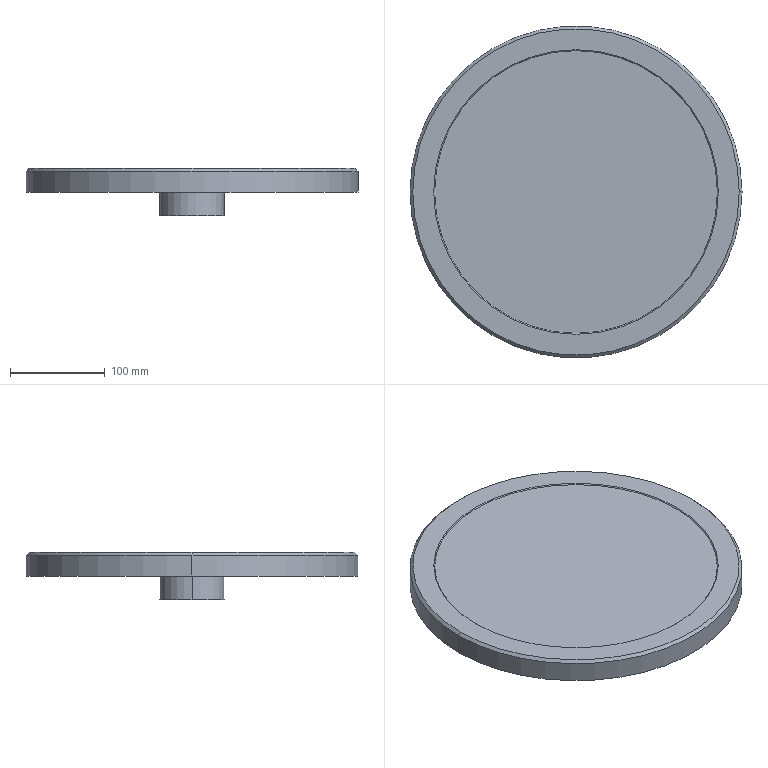Part | SolidWorks | features ICE 2, Chamfer 1, Extrusion 1, Fillet 1 | 1 solid | 14 faces | box 350 x 350 x 50 mm | volume 2420950 mm3 | cone 4 | cylinder 4 | plane 4 | torus 2 | commonest cylinder face diameters 68 x2 350 x2
STEP:
#1=CARTESIAN_POINT('',(172.,0.,50.));
#2=VERTEX_POINT('',#1);
#3=CARTESIAN_POINT('',(-172.,0.,50.));
#4=VERTEX_POINT('',#3);
#5=CARTESIAN_POINT('',(0.,0.,50.));
#6=DIRECTION('',(0.,0.,1.));
#7=DIRECTION('',(1.,0.,0.));
#8=AXIS2_PLACEMENT_3D('',#5,#6,#7);
#9=CIRCLE('',#8,172.);
#10=EDGE_CURVE('',#2,#4,#9,.T.);
#11=ORIENTED_EDGE('',*,*,#10,.F.);
#12=CARTESIAN_POINT('',(175.,0.,47.));
#13=VERTEX_POINT('',#12);
#14=CARTESIAN_POINT('',(172.,0.,50.));
#15=DIRECTION('',(0.7071,0.,-0.7071));
#16=VECTOR('',#15,1000.);
#17=LINE('',#14,#16);
#18=EDGE_CURVE('',#2,#13,#17,.T.);
#19=ORIENTED_EDGE('',*,*,#18,.T.);
#20=CARTESIAN_POINT('',(-175.,0.,47.));
#21=VERTEX_POINT('',#20);
#22=CARTESIAN_POINT('',(0.,0.,47.));
#23=DIRECTION('',(0.,0.,-1.));
#24=DIRECTION('',(1.,0.,0.));
#25=AXIS2_PLACEMENT_3D('',#22,#23,#24);
#26=CIRCLE('',#25,175.);
#27=EDGE_CURVE('',#21,#13,#26,.T.);
#28=ORIENTED_EDGE('',*,*,#27,.F.);
#29=CARTESIAN_POINT('',(-172.,0.,50.));
#30=DIRECTION('',(-0.7071,0.,-0.7071));
#31=VECTOR('',#30,1000.);
#32=LINE('',#29,#31);
#33=EDGE_CURVE('',#4,#21,#32,.T.);
#34=ORIENTED_EDGE('',*,*,#33,.F.);
#35=EDGE_LOOP('',(#11,#19,#28,#34));
#36=FACE_OUTER_BOUND('',#35,.T.);
#37=CARTESIAN_POINT('',(0.,0.,50.));
#38=DIRECTION('',(0.,0.,-1.));
#39=DIRECTION('',(-1.,0.,0.));
#40=AXIS2_PLACEMENT_3D('',#37,#38,#39);
#41=CONICAL_SURFACE('',#40,172.,0.7854);
#42=ADVANCED_FACE('',(#36),#41,.T.);
#43=CARTESIAN_POINT('',(-34.5,0.,25.));
#44=VERTEX_POINT('',#43);
#45=CARTESIAN_POINT('',(34.5,0.,25.));
#46=VERTEX_POINT('',#45);
#47=CARTESIAN_POINT('',(0.,0.,25.));
#48=DIRECTION('',(0.,0.,1.));
#49=DIRECTION('',(1.,0.,0.));
#50=AXIS2_PLACEMENT_3D('',#47,#48,#49);
#51=CIRCLE('',#50,34.5);
#52=EDGE_CURVE('',#44,#46,#51,.T.);
#53=ORIENTED_EDGE('',*,*,#52,.F.);
#54=CARTESIAN_POINT('',(-34.,0.,24.5));
#55=VERTEX_POINT('',#54);
#56=CARTESIAN_POINT('',(-34.5,0.,24.5));
#57=DIRECTION('',(0.,1.,0.));
#58=DIRECTION('',(-1.,0.,0.));
#59=AXIS2_PLACEMENT_3D('',#56,#57,#58);
#60=CIRCLE('',#59,0.5);
#61=EDGE_CURVE('',#44,#55,#60,.T.);
#62=ORIENTED_EDGE('',*,*,#61,.T.);
#63=CARTESIAN_POINT('',(34.,0.,24.5));
#64=VERTEX_POINT('',#63);
#65=CARTESIAN_POINT('',(0.,0.,24.5));
#66=DIRECTION('',(0.,0.,-1.));
#67=DIRECTION('',(1.,0.,0.));
#68=AXIS2_PLACEMENT_3D('',#65,#66,#67);
#69=CIRCLE('',#68,34.);
#70=EDGE_CURVE('',#64,#55,#69,.T.);
#71=ORIENTED_EDGE('',*,*,#70,.F.);
#72=CARTESIAN_POINT('',(34.5,0.,24.5));
#73=DIRECTION('',(0.,-1.,0.));
#74=DIRECTION('',(0.,0.,-1.));
#75=AXIS2_PLACEMENT_3D('',#72,#73,#74);
#76=CIRCLE('',#75,0.5);
#77=EDGE_CURVE('',#46,#64,#76,.T.);
#78=ORIENTED_EDGE('',*,*,#77,.F.);
#79=EDGE_LOOP('',(#53,#62,#71,#78));
#80=FACE_OUTER_BOUND('',#79,.T.);
#81=CARTESIAN_POINT('',(0.,0.,24.5));
#82=DIRECTION('',(0.,0.,1.));
#83=DIRECTION('',(1.,0.,0.));
#84=AXIS2_PLACEMENT_3D('',#81,#82,#83);
#85=TOROIDAL_SURFACE('',#84,34.5,0.5);
#86=ADVANCED_FACE('',(#80),#85,.F.);
#87=CARTESIAN_POINT('',(-149.,0.,49.));
#88=VERTEX_POINT('',#87);
#89=CARTESIAN_POINT('',(149.,0.,49.));
#90=VERTEX_POINT('',#89);
#91=CARTESIAN_POINT('',(0.,0.,49.));
#92=DIRECTION('',(0.,0.,1.));
#93=DIRECTION('',(1.,0.,0.));
#94=AXIS2_PLACEMENT_3D('',#91,#92,#93);
#95=CIRCLE('',#94,149.);
#96=EDGE_CURVE('',#88,#90,#95,.T.);
#97=ORIENTED_EDGE('',*,*,#96,.F.);
#98=CARTESIAN_POINT('',(-150.,0.,50.));
#99=VERTEX_POINT('',#98);
#100=CARTESIAN_POINT('',(-150.,0.,50.));
#101=DIRECTION('',(-0.7071,0.,0.7071));
#102=VECTOR('',#101,1000.);
#103=LINE('',#100,#102);
#104=EDGE_CURVE('',#88,#99,#103,.T.);
#105=ORIENTED_EDGE('',*,*,#104,.T.);
#106=CARTESIAN_POINT('',(150.,0.,50.));
#107=VERTEX_POINT('',#106);
#108=CARTESIAN_POINT('',(0.,0.,50.));
#109=DIRECTION('',(0.,0.,1.));
#110=DIRECTION('',(1.,0.,0.));
#111=AXIS2_PLACEMENT_3D('',#108,#109,#110);
#112=CIRCLE('',#111,150.);
#113=EDGE_CURVE('',#99,#107,#112,.T.);
#114=ORIENTED_EDGE('',*,*,#113,.T.);
#115=CARTESIAN_POINT('',(150.,0.,50.));
#116=DIRECTION('',(0.7071,0.,0.7071));
#117=VECTOR('',#116,1000.);
#118=LINE('',#115,#117);
#119=EDGE_CURVE('',#90,#107,#118,.T.);
#120=ORIENTED_EDGE('',*,*,#119,.F.);
#121=EDGE_LOOP('',(#97,#105,#114,#120));
#122=FACE_OUTER_BOUND('',#121,.T.);
#123=CARTESIAN_POINT('',(0.,0.,50.));
#124=DIRECTION('',(0.,0.,1.));
#125=DIRECTION('',(1.,0.,0.));
#126=AXIS2_PLACEMENT_3D('',#123,#124,#125);
#127=CONICAL_SURFACE('',#126,150.,0.7854);
#128=ADVANCED_FACE('',(#122),#127,.F.);
#129=CARTESIAN_POINT('',(175.,0.,25.));
#130=VERTEX_POINT('',#129);
#131=CARTESIAN_POINT('',(-175.,0.,25.));
#132=VERTEX_POINT('',#131);
#133=CARTESIAN_POINT('',(0.,0.,25.));
#134=DIRECTION('',(0.,0.,1.));
#135=DIRECTION('',(1.,0.,0.));
#136=AXIS2_PLACEMENT_3D('',#133,#134,#135);
#137=CIRCLE('',#136,175.);
#138=EDGE_CURVE('',#130,#132,#137,.T.);
#139=ORIENTED_EDGE('',*,*,#138,.T.);
#140=CARTESIAN_POINT('',(-175.,0.,25.));
#141=DIRECTION('',(0.,0.,1.));
#142=VECTOR('',#141,1000.);
#143=LINE('',#140,#142);
#144=EDGE_CURVE('',#132,#21,#143,.T.);
#145=ORIENTED_EDGE('',*,*,#144,.T.);
#146=ORIENTED_EDGE('',*,*,#27,.T.);
#147=CARTESIAN_POINT('',(175.,0.,25.));
#148=DIRECTION('',(0.,0.,1.));
#149=VECTOR('',#148,1000.);
#150=LINE('',#147,#149);
#151=EDGE_CURVE('',#130,#13,#150,.T.);
#152=ORIENTED_EDGE('',*,*,#151,.F.);
#153=EDGE_LOOP('',(#139,#145,#146,#152));
#154=FACE_OUTER_BOUND('',#153,.T.);
#155=CARTESIAN_POINT('',(0.,0.,25.));
#156=DIRECTION('',(0.,0.,1.));
#157=DIRECTION('',(1.,0.,0.));
#158=AXIS2_PLACEMENT_3D('',#155,#156,#157);
#159=CYLINDRICAL_SURFACE('',#158,175.);
#160=ADVANCED_FACE('',(#154),#159,.T.);
#161=CARTESIAN_POINT('',(0.,0.,24.5));
#162=DIRECTION('',(0.,0.,-1.));
#163=DIRECTION('',(1.,0.,0.));
#164=AXIS2_PLACEMENT_3D('',#161,#162,#163);
#165=CIRCLE('',#164,34.);
#166=EDGE_CURVE('',#55,#64,#165,.T.);
#167=ORIENTED_EDGE('',*,*,#166,.T.);
#168=CARTESIAN_POINT('',(34.,0.,0.));
#169=VERTEX_POINT('',#168);
#170=CARTESIAN_POINT('',(34.,0.,50.));
#171=DIRECTION('',(0.,0.,-1.));
#172=VECTOR('',#171,1000.);
#173=LINE('',#170,#172);
#174=EDGE_CURVE('',#64,#169,#173,.T.);
#175=ORIENTED_EDGE('',*,*,#174,.T.);
#176=CARTESIAN_POINT('',(-34.,0.,0.));
#177=VERTEX_POINT('',#176);
#178=CARTESIAN_POINT('',(0.,0.,0.));
#179=DIRECTION('',(0.,0.,1.));
#180=DIRECTION('',(1.,0.,0.));
#181=AXIS2_PLACEMENT_3D('',#178,#179,#180);
#182=CIRCLE('',#181,34.);
#183=EDGE_CURVE('',#169,#177,#182,.T.);
#184=ORIENTED_EDGE('',*,*,#183,.T.);
#185=CARTESIAN_POINT('',(-34.,0.,50.));
#186=DIRECTION('',(0.,0.,-1.));
#187=VECTOR('',#186,1000.);
#188=LINE('',#185,#187);
#189=EDGE_CURVE('',#55,#177,#188,.T.);
#190=ORIENTED_EDGE('',*,*,#189,.F.);
#191=EDGE_LOOP('',(#167,#175,#184,#190));
#192=FACE_OUTER_BOUND('',#191,.T.);
#193=CARTESIAN_POINT('',(0.,0.,50.));
#194=DIRECTION('',(0.,0.,-1.));
#195=DIRECTION('',(-1.,0.,0.));
#196=AXIS2_PLACEMENT_3D('',#193,#194,#195);
#197=CYLINDRICAL_SURFACE('',#196,34.);
#198=ADVANCED_FACE('',(#192),#197,.T.);
#199=ORIENTED_EDGE('',*,*,#174,.F.);
#200=ORIENTED_EDGE('',*,*,#70,.T.);
#201=ORIENTED_EDGE('',*,*,#189,.T.);
#202=CARTESIAN_POINT('',(0.,0.,0.));
#203=DIRECTION('',(0.,0.,1.));
#204=DIRECTION('',(1.,0.,0.));
#205=AXIS2_PLACEMENT_3D('',#202,#203,#204);
#206=CIRCLE('',#205,34.);
#207=EDGE_CURVE('',#177,#169,#206,.T.);
#208=ORIENTED_EDGE('',*,*,#207,.T.);
#209=EDGE_LOOP('',(#199,#200,#201,#208));
#210=FACE_OUTER_BOUND('',#209,.T.);
#211=CARTESIAN_POINT('',(0.,0.,50.));
#212=DIRECTION('',(0.,0.,-1.));
#213=DIRECTION('',(-1.,0.,0.));
#214=AXIS2_PLACEMENT_3D('',#211,#212,#213);
#215=CYLINDRICAL_SURFACE('',#214,34.);
#216=ADVANCED_FACE('',(#210),#215,.T.);
#217=ORIENTED_EDGE('',*,*,#207,.F.);
#218=ORIENTED_EDGE('',*,*,#183,.F.);
#219=EDGE_LOOP('',(#217,#218));
#220=FACE_OUTER_BOUND('',#219,.T.);
#221=CARTESIAN_POINT('',(0.,0.,0.));
#222=DIRECTION('',(0.,0.,1.));
#223=DIRECTION('',(1.,0.,0.));
#224=AXIS2_PLACEMENT_3D('',#221,#222,#223);
#225=PLANE('',#224);
#226=ADVANCED_FACE('',(#220),#225,.F.);
#227=ORIENTED_EDGE('',*,*,#144,.F.);
#228=CARTESIAN_POINT('',(0.,0.,25.));
#229=DIRECTION('',(0.,0.,1.));
#230=DIRECTION('',(1.,0.,0.));
#231=AXIS2_PLACEMENT_3D('',#228,#229,#230);
#232=CIRCLE('',#231,175.);
#233=EDGE_CURVE('',#132,#130,#232,.T.);
#234=ORIENTED_EDGE('',*,*,#233,.T.);
#235=ORIENTED_EDGE('',*,*,#151,.T.);
#236=CARTESIAN_POINT('',(0.,0.,47.));
#237=DIRECTION('',(0.,0.,-1.));
#238=DIRECTION('',(1.,0.,0.));
#239=AXIS2_PLACEMENT_3D('',#236,#237,#238);
#240=CIRCLE('',#239,175.);
#241=EDGE_CURVE('',#13,#21,#240,.T.);
#242=ORIENTED_EDGE('',*,*,#241,.T.);
#243=EDGE_LOOP('',(#227,#234,#235,#242));
#244=FACE_OUTER_BOUND('',#243,.T.);
#245=CARTESIAN_POINT('',(0.,0.,25.));
#246=DIRECTION('',(0.,0.,1.));
#247=DIRECTION('',(1.,0.,0.));
#248=AXIS2_PLACEMENT_3D('',#245,#246,#247);
#249=CYLINDRICAL_SURFACE('',#248,175.);
#250=ADVANCED_FACE('',(#244),#249,.T.);
#251=CARTESIAN_POINT('',(0.,0.,25.));
#252=DIRECTION('',(0.,0.,1.));
#253=DIRECTION('',(1.,0.,0.));
#254=AXIS2_PLACEMENT_3D('',#251,#252,#253);
#255=CIRCLE('',#254,34.5);
#256=EDGE_CURVE('',#46,#44,#255,.T.);
#257=ORIENTED_EDGE('',*,*,#256,.T.);
#258=ORIENTED_EDGE('',*,*,#52,.T.);
#259=EDGE_LOOP('',(#257,#258));
#260=FACE_BOUND('',#259,.T.);
#261=ORIENTED_EDGE('',*,*,#138,.F.);
#262=ORIENTED_EDGE('',*,*,#233,.F.);
#263=EDGE_LOOP('',(#261,#262));
#264=FACE_OUTER_BOUND('',#263,.T.);
#265=CARTESIAN_POINT('',(0.,0.,25.));
#266=DIRECTION('',(0.,0.,1.));
#267=DIRECTION('',(1.,0.,0.));
#268=AXIS2_PLACEMENT_3D('',#265,#266,#267);
#269=PLANE('',#268);
#270=ADVANCED_FACE('',(#260,#264),#269,.F.);
#271=CARTESIAN_POINT('',(0.,0.,50.));
#272=DIRECTION('',(0.,0.,1.));
#273=DIRECTION('',(1.,0.,0.));
#274=AXIS2_PLACEMENT_3D('',#271,#272,#273);
#275=CIRCLE('',#274,172.);
#276=EDGE_CURVE('',#4,#2,#275,.T.);
#277=ORIENTED_EDGE('',*,*,#276,.T.);
#278=ORIENTED_EDGE('',*,*,#10,.T.);
#279=EDGE_LOOP('',(#277,#278));
#280=FACE_OUTER_BOUND('',#279,.T.);
#281=CARTESIAN_POINT('',(0.,0.,50.));
#282=DIRECTION('',(0.,0.,1.));
#283=DIRECTION('',(1.,0.,0.));
#284=AXIS2_PLACEMENT_3D('',#281,#282,#283);
#285=CIRCLE('',#284,150.);
#286=EDGE_CURVE('',#107,#99,#285,.T.);
#287=ORIENTED_EDGE('',*,*,#286,.F.);
#288=ORIENTED_EDGE('',*,*,#113,.F.);
#289=EDGE_LOOP('',(#287,#288));
#290=FACE_BOUND('',#289,.T.);
#291=CARTESIAN_POINT('',(0.,0.,50.));
#292=DIRECTION('',(0.,0.,1.));
#293=DIRECTION('',(1.,0.,0.));
#294=AXIS2_PLACEMENT_3D('',#291,#292,#293);
#295=PLANE('',#294);
#296=ADVANCED_FACE('',(#280,#290),#295,.T.);
#297=ORIENTED_EDGE('',*,*,#104,.F.);
#298=CARTESIAN_POINT('',(0.,0.,49.));
#299=DIRECTION('',(0.,0.,1.));
#300=DIRECTION('',(1.,0.,0.));
#301=AXIS2_PLACEMENT_3D('',#298,#299,#300);
#302=CIRCLE('',#301,149.);
#303=EDGE_CURVE('',#90,#88,#302,.T.);
#304=ORIENTED_EDGE('',*,*,#303,.F.);
#305=ORIENTED_EDGE('',*,*,#119,.T.);
#306=ORIENTED_EDGE('',*,*,#286,.T.);
#307=EDGE_LOOP('',(#297,#304,#305,#306));
#308=FACE_OUTER_BOUND('',#307,.T.);
#309=CARTESIAN_POINT('',(0.,0.,50.));
#310=DIRECTION('',(0.,0.,1.));
#311=DIRECTION('',(1.,0.,0.));
#312=AXIS2_PLACEMENT_3D('',#309,#310,#311);
#313=CONICAL_SURFACE('',#312,150.,0.7854);
#314=ADVANCED_FACE('',(#308),#313,.F.);
#315=ORIENTED_EDGE('',*,*,#303,.T.);
#316=ORIENTED_EDGE('',*,*,#96,.T.);
#317=EDGE_LOOP('',(#315,#316));
#318=FACE_OUTER_BOUND('',#317,.T.);
#319=CARTESIAN_POINT('',(0.,0.,49.));
#320=DIRECTION('',(0.,0.,1.));
#321=DIRECTION('',(1.,0.,0.));
#322=AXIS2_PLACEMENT_3D('',#319,#320,#321);
#323=PLANE('',#322);
#324=ADVANCED_FACE('',(#318),#323,.T.);
#325=ORIENTED_EDGE('',*,*,#61,.F.);
#326=ORIENTED_EDGE('',*,*,#256,.F.);
#327=ORIENTED_EDGE('',*,*,#77,.T.);
#328=ORIENTED_EDGE('',*,*,#166,.F.);
#329=EDGE_LOOP('',(#325,#326,#327,#328));
#330=FACE_OUTER_BOUND('',#329,.T.);
#331=CARTESIAN_POINT('',(0.,0.,24.5));
#332=DIRECTION('',(0.,0.,1.));
#333=DIRECTION('',(1.,0.,0.));
#334=AXIS2_PLACEMENT_3D('',#331,#332,#333);
#335=TOROIDAL_SURFACE('',#334,34.5,0.5);
#336=ADVANCED_FACE('',(#330),#335,.F.);
#337=ORIENTED_EDGE('',*,*,#18,.F.);
#338=ORIENTED_EDGE('',*,*,#276,.F.);
#339=ORIENTED_EDGE('',*,*,#33,.T.);
#340=ORIENTED_EDGE('',*,*,#241,.F.);
#341=EDGE_LOOP('',(#337,#338,#339,#340));
#342=FACE_OUTER_BOUND('',#341,.T.);
#343=CARTESIAN_POINT('',(0.,0.,50.));
#344=DIRECTION('',(0.,0.,-1.));
#345=DIRECTION('',(-1.,0.,0.));
#346=AXIS2_PLACEMENT_3D('',#343,#344,#345);
#347=CONICAL_SURFACE('',#346,172.,0.7854);
#348=ADVANCED_FACE('',(#342),#347,.T.);
#349=CLOSED_SHELL('',(#42,#86,#128,#160,#198,#216,#226,#250,#270,#296,#314,#324,#336,#348));
#350=MANIFOLD_SOLID_BREP('',#349);
#351=CARTESIAN_POINT('',(0.,0.,0.));
#352=DIRECTION('',(0.,0.,1.));
#353=DIRECTION('',(1.,0.,0.));
#354=AXIS2_PLACEMENT_3D('',#351,#352,#353);
#355=(LENGTH_UNIT()NAMED_UNIT(*)SI_UNIT(.MILLI.,.METRE.));
#356=UNCERTAINTY_MEASURE_WITH_UNIT(LENGTH_MEASURE(0.00001),#355,'','');
#357=(NAMED_UNIT(*)PLANE_ANGLE_UNIT()SI_UNIT($,.RADIAN.));
#358=(NAMED_UNIT(*)SI_UNIT($,.STERADIAN.)SOLID_ANGLE_UNIT());
#359=(GEOMETRIC_REPRESENTATION_CONTEXT(3)GLOBAL_UNCERTAINTY_ASSIGNED_CONTEXT((#356))GLOBAL_UNIT_ASSIGNED_CONTEXT((#355,#357,#358))REPRESENTATION_CONTEXT('',''));
#360=ADVANCED_BREP_SHAPE_REPRESENTATION('',(#350,#354),#359);